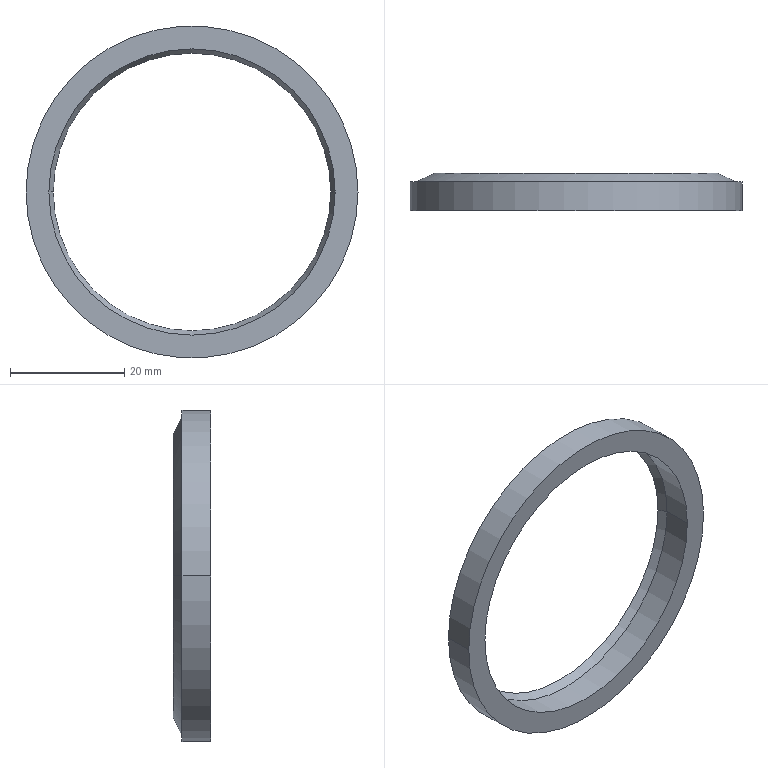Part | SolidWorks | features Revolution 1 | 1 solid | 11 faces | box 58 x 6.5 x 58 mm | volume 3817 mm3 | cone 4 | cylinder 4 | plane 3 | commonest cylinder face diameters 50 x2 58 x2
STEP:
#1=CARTESIAN_POINT('',(-24.25,6.5,0.));
#2=VERTEX_POINT('',#1);
#3=CARTESIAN_POINT('',(24.25,6.5,0.));
#4=VERTEX_POINT('',#3);
#5=CARTESIAN_POINT('',(0.,6.5,0.));
#6=DIRECTION('',(0.,-1.,0.));
#7=DIRECTION('',(1.,0.,0.));
#8=AXIS2_PLACEMENT_3D('',#5,#6,#7);
#9=CIRCLE('',#8,24.25);
#10=EDGE_CURVE('',#2,#4,#9,.T.);
#11=ORIENTED_EDGE('',*,*,#10,.F.);
#12=CARTESIAN_POINT('',(-25.,5.,0.));
#13=VERTEX_POINT('',#12);
#14=CARTESIAN_POINT('',(-24.25,6.5,0.));
#15=DIRECTION('',(-0.4472,-0.8944,0.));
#16=VECTOR('',#15,1000.);
#17=LINE('',#14,#16);
#18=EDGE_CURVE('',#2,#13,#17,.T.);
#19=ORIENTED_EDGE('',*,*,#18,.T.);
#20=CARTESIAN_POINT('',(25.,5.,0.));
#21=VERTEX_POINT('',#20);
#22=CARTESIAN_POINT('',(0.,5.,0.));
#23=DIRECTION('',(0.,-1.,0.));
#24=DIRECTION('',(1.,0.,0.));
#25=AXIS2_PLACEMENT_3D('',#22,#23,#24);
#26=CIRCLE('',#25,25.);
#27=EDGE_CURVE('',#13,#21,#26,.T.);
#28=ORIENTED_EDGE('',*,*,#27,.T.);
#29=CARTESIAN_POINT('',(24.25,6.5,0.));
#30=DIRECTION('',(0.4472,-0.8944,0.));
#31=VECTOR('',#30,1000.);
#32=LINE('',#29,#31);
#33=EDGE_CURVE('',#4,#21,#32,.T.);
#34=ORIENTED_EDGE('',*,*,#33,.F.);
#35=EDGE_LOOP('',(#11,#19,#28,#34));
#36=FACE_OUTER_BOUND('',#35,.T.);
#37=CARTESIAN_POINT('',(0.,6.5,0.));
#38=DIRECTION('',(0.,-1.,0.));
#39=DIRECTION('',(1.,0.,0.));
#40=AXIS2_PLACEMENT_3D('',#37,#38,#39);
#41=CONICAL_SURFACE('',#40,24.25,0.4636);
#42=ADVANCED_FACE('',(#36),#41,.F.);
#43=CARTESIAN_POINT('',(24.75,6.5,0.));
#44=VERTEX_POINT('',#43);
#45=CARTESIAN_POINT('',(-24.75,6.5,0.));
#46=VERTEX_POINT('',#45);
#47=CARTESIAN_POINT('',(0.,6.5,0.));
#48=DIRECTION('',(0.,-1.,0.));
#49=DIRECTION('',(1.,0.,0.));
#50=AXIS2_PLACEMENT_3D('',#47,#48,#49);
#51=CIRCLE('',#50,24.75);
#52=EDGE_CURVE('',#44,#46,#51,.T.);
#53=ORIENTED_EDGE('',*,*,#52,.T.);
#54=CARTESIAN_POINT('',(-28.,5.,0.));
#55=VERTEX_POINT('',#54);
#56=CARTESIAN_POINT('',(-28.,5.,0.));
#57=DIRECTION('',(-0.908,-0.4191,0.));
#58=VECTOR('',#57,1000.);
#59=LINE('',#56,#58);
#60=EDGE_CURVE('',#46,#55,#59,.T.);
#61=ORIENTED_EDGE('',*,*,#60,.T.);
#62=CARTESIAN_POINT('',(28.,5.,0.));
#63=VERTEX_POINT('',#62);
#64=CARTESIAN_POINT('',(0.,5.,0.));
#65=DIRECTION('',(0.,-1.,0.));
#66=DIRECTION('',(1.,0.,0.));
#67=AXIS2_PLACEMENT_3D('',#64,#65,#66);
#68=CIRCLE('',#67,28.);
#69=EDGE_CURVE('',#63,#55,#68,.T.);
#70=ORIENTED_EDGE('',*,*,#69,.F.);
#71=CARTESIAN_POINT('',(28.,5.,0.));
#72=DIRECTION('',(0.908,-0.4191,0.));
#73=VECTOR('',#72,1000.);
#74=LINE('',#71,#73);
#75=EDGE_CURVE('',#44,#63,#74,.T.);
#76=ORIENTED_EDGE('',*,*,#75,.F.);
#77=EDGE_LOOP('',(#53,#61,#70,#76));
#78=FACE_OUTER_BOUND('',#77,.T.);
#79=CARTESIAN_POINT('',(0.,5.,0.));
#80=DIRECTION('',(0.,-1.,0.));
#81=DIRECTION('',(1.,0.,0.));
#82=AXIS2_PLACEMENT_3D('',#79,#80,#81);
#83=CONICAL_SURFACE('',#82,28.,1.138);
#84=ADVANCED_FACE('',(#78),#83,.T.);
#85=CARTESIAN_POINT('',(29.,5.,0.));
#86=VERTEX_POINT('',#85);
#87=CARTESIAN_POINT('',(-29.,5.,0.));
#88=VERTEX_POINT('',#87);
#89=CARTESIAN_POINT('',(0.,5.,0.));
#90=DIRECTION('',(0.,-1.,0.));
#91=DIRECTION('',(1.,0.,0.));
#92=AXIS2_PLACEMENT_3D('',#89,#90,#91);
#93=CIRCLE('',#92,29.);
#94=EDGE_CURVE('',#86,#88,#93,.T.);
#95=ORIENTED_EDGE('',*,*,#94,.T.);
#96=CARTESIAN_POINT('',(-29.,0.,0.));
#97=VERTEX_POINT('',#96);
#98=CARTESIAN_POINT('',(-29.,-1000.,0.));
#99=DIRECTION('',(0.,-1.,0.));
#100=VECTOR('',#99,1000.);
#101=LINE('',#98,#100);
#102=EDGE_CURVE('',#88,#97,#101,.T.);
#103=ORIENTED_EDGE('',*,*,#102,.T.);
#104=CARTESIAN_POINT('',(29.,0.,0.));
#105=VERTEX_POINT('',#104);
#106=CARTESIAN_POINT('',(0.,0.,0.));
#107=DIRECTION('',(0.,-1.,0.));
#108=DIRECTION('',(1.,0.,0.));
#109=AXIS2_PLACEMENT_3D('',#106,#107,#108);
#110=CIRCLE('',#109,29.);
#111=EDGE_CURVE('',#105,#97,#110,.T.);
#112=ORIENTED_EDGE('',*,*,#111,.F.);
#113=CARTESIAN_POINT('',(29.,-1000.,0.));
#114=DIRECTION('',(0.,-1.,0.));
#115=VECTOR('',#114,1000.);
#116=LINE('',#113,#115);
#117=EDGE_CURVE('',#86,#105,#116,.T.);
#118=ORIENTED_EDGE('',*,*,#117,.F.);
#119=EDGE_LOOP('',(#95,#103,#112,#118));
#120=FACE_OUTER_BOUND('',#119,.T.);
#121=CARTESIAN_POINT('',(0.,-1000.,0.));
#122=DIRECTION('',(0.,-1.,0.));
#123=DIRECTION('',(1.,0.,0.));
#124=AXIS2_PLACEMENT_3D('',#121,#122,#123);
#125=CYLINDRICAL_SURFACE('',#124,29.);
#126=ADVANCED_FACE('',(#120),#125,.T.);
#127=ORIENTED_EDGE('',*,*,#27,.F.);
#128=CARTESIAN_POINT('',(-25.,0.,0.));
#129=VERTEX_POINT('',#128);
#130=CARTESIAN_POINT('',(-25.,-1000.,0.));
#131=DIRECTION('',(0.,-1.,0.));
#132=VECTOR('',#131,1000.);
#133=LINE('',#130,#132);
#134=EDGE_CURVE('',#13,#129,#133,.T.);
#135=ORIENTED_EDGE('',*,*,#134,.T.);
#136=CARTESIAN_POINT('',(25.,0.,0.));
#137=VERTEX_POINT('',#136);
#138=CARTESIAN_POINT('',(0.,0.,0.));
#139=DIRECTION('',(0.,-1.,0.));
#140=DIRECTION('',(1.,0.,0.));
#141=AXIS2_PLACEMENT_3D('',#138,#139,#140);
#142=CIRCLE('',#141,25.);
#143=EDGE_CURVE('',#129,#137,#142,.T.);
#144=ORIENTED_EDGE('',*,*,#143,.T.);
#145=CARTESIAN_POINT('',(25.,-1000.,0.));
#146=DIRECTION('',(0.,-1.,0.));
#147=VECTOR('',#146,1000.);
#148=LINE('',#145,#147);
#149=EDGE_CURVE('',#21,#137,#148,.T.);
#150=ORIENTED_EDGE('',*,*,#149,.F.);
#151=EDGE_LOOP('',(#127,#135,#144,#150));
#152=FACE_OUTER_BOUND('',#151,.T.);
#153=CARTESIAN_POINT('',(0.,-1000.,0.));
#154=DIRECTION('',(0.,-1.,0.));
#155=DIRECTION('',(1.,0.,0.));
#156=AXIS2_PLACEMENT_3D('',#153,#154,#155);
#157=CYLINDRICAL_SURFACE('',#156,25.);
#158=ADVANCED_FACE('',(#152),#157,.F.);
#159=ORIENTED_EDGE('',*,*,#134,.F.);
#160=CARTESIAN_POINT('',(0.,5.,0.));
#161=DIRECTION('',(0.,-1.,0.));
#162=DIRECTION('',(1.,0.,0.));
#163=AXIS2_PLACEMENT_3D('',#160,#161,#162);
#164=CIRCLE('',#163,25.);
#165=EDGE_CURVE('',#21,#13,#164,.T.);
#166=ORIENTED_EDGE('',*,*,#165,.F.);
#167=ORIENTED_EDGE('',*,*,#149,.T.);
#168=CARTESIAN_POINT('',(0.,0.,0.));
#169=DIRECTION('',(0.,-1.,0.));
#170=DIRECTION('',(1.,0.,0.));
#171=AXIS2_PLACEMENT_3D('',#168,#169,#170);
#172=CIRCLE('',#171,25.);
#173=EDGE_CURVE('',#137,#129,#172,.T.);
#174=ORIENTED_EDGE('',*,*,#173,.T.);
#175=EDGE_LOOP('',(#159,#166,#167,#174));
#176=FACE_OUTER_BOUND('',#175,.T.);
#177=CARTESIAN_POINT('',(0.,-1000.,0.));
#178=DIRECTION('',(0.,-1.,0.));
#179=DIRECTION('',(1.,0.,0.));
#180=AXIS2_PLACEMENT_3D('',#177,#178,#179);
#181=CYLINDRICAL_SURFACE('',#180,25.);
#182=ADVANCED_FACE('',(#176),#181,.F.);
#183=ORIENTED_EDGE('',*,*,#111,.T.);
#184=CARTESIAN_POINT('',(0.,0.,0.));
#185=DIRECTION('',(0.,-1.,0.));
#186=DIRECTION('',(1.,0.,0.));
#187=AXIS2_PLACEMENT_3D('',#184,#185,#186);
#188=CIRCLE('',#187,29.);
#189=EDGE_CURVE('',#97,#105,#188,.T.);
#190=ORIENTED_EDGE('',*,*,#189,.T.);
#191=EDGE_LOOP('',(#183,#190));
#192=FACE_OUTER_BOUND('',#191,.T.);
#193=ORIENTED_EDGE('',*,*,#173,.F.);
#194=ORIENTED_EDGE('',*,*,#143,.F.);
#195=EDGE_LOOP('',(#193,#194));
#196=FACE_BOUND('',#195,.T.);
#197=CARTESIAN_POINT('',(25.,0.,0.));
#198=DIRECTION('',(0.,-1.,0.));
#199=DIRECTION('',(1.,0.,0.));
#200=AXIS2_PLACEMENT_3D('',#197,#198,#199);
#201=PLANE('',#200);
#202=ADVANCED_FACE('',(#192,#196),#201,.T.);
#203=ORIENTED_EDGE('',*,*,#102,.F.);
#204=CARTESIAN_POINT('',(0.,5.,0.));
#205=DIRECTION('',(0.,-1.,0.));
#206=DIRECTION('',(1.,0.,0.));
#207=AXIS2_PLACEMENT_3D('',#204,#205,#206);
#208=CIRCLE('',#207,29.);
#209=EDGE_CURVE('',#88,#86,#208,.T.);
#210=ORIENTED_EDGE('',*,*,#209,.T.);
#211=ORIENTED_EDGE('',*,*,#117,.T.);
#212=ORIENTED_EDGE('',*,*,#189,.F.);
#213=EDGE_LOOP('',(#203,#210,#211,#212));
#214=FACE_OUTER_BOUND('',#213,.T.);
#215=CARTESIAN_POINT('',(0.,-1000.,0.));
#216=DIRECTION('',(0.,-1.,0.));
#217=DIRECTION('',(1.,0.,0.));
#218=AXIS2_PLACEMENT_3D('',#215,#216,#217);
#219=CYLINDRICAL_SURFACE('',#218,29.);
#220=ADVANCED_FACE('',(#214),#219,.T.);
#221=ORIENTED_EDGE('',*,*,#69,.T.);
#222=CARTESIAN_POINT('',(0.,5.,0.));
#223=DIRECTION('',(0.,-1.,0.));
#224=DIRECTION('',(1.,0.,0.));
#225=AXIS2_PLACEMENT_3D('',#222,#223,#224);
#226=CIRCLE('',#225,28.);
#227=EDGE_CURVE('',#55,#63,#226,.T.);
#228=ORIENTED_EDGE('',*,*,#227,.T.);
#229=EDGE_LOOP('',(#221,#228));
#230=FACE_BOUND('',#229,.T.);
#231=ORIENTED_EDGE('',*,*,#94,.F.);
#232=ORIENTED_EDGE('',*,*,#209,.F.);
#233=EDGE_LOOP('',(#231,#232));
#234=FACE_OUTER_BOUND('',#233,.T.);
#235=CARTESIAN_POINT('',(29.,5.,0.));
#236=DIRECTION('',(0.,1.,0.));
#237=DIRECTION('',(-1.,0.,0.));
#238=AXIS2_PLACEMENT_3D('',#235,#236,#237);
#239=PLANE('',#238);
#240=ADVANCED_FACE('',(#230,#234),#239,.T.);
#241=ORIENTED_EDGE('',*,*,#60,.F.);
#242=CARTESIAN_POINT('',(0.,6.5,0.));
#243=DIRECTION('',(0.,-1.,0.));
#244=DIRECTION('',(1.,0.,0.));
#245=AXIS2_PLACEMENT_3D('',#242,#243,#244);
#246=CIRCLE('',#245,24.75);
#247=EDGE_CURVE('',#46,#44,#246,.T.);
#248=ORIENTED_EDGE('',*,*,#247,.T.);
#249=ORIENTED_EDGE('',*,*,#75,.T.);
#250=ORIENTED_EDGE('',*,*,#227,.F.);
#251=EDGE_LOOP('',(#241,#248,#249,#250));
#252=FACE_OUTER_BOUND('',#251,.T.);
#253=CARTESIAN_POINT('',(0.,5.,0.));
#254=DIRECTION('',(0.,-1.,0.));
#255=DIRECTION('',(1.,0.,0.));
#256=AXIS2_PLACEMENT_3D('',#253,#254,#255);
#257=CONICAL_SURFACE('',#256,28.,1.138);
#258=ADVANCED_FACE('',(#252),#257,.T.);
#259=CARTESIAN_POINT('',(0.,6.5,0.));
#260=DIRECTION('',(0.,-1.,0.));
#261=DIRECTION('',(1.,0.,0.));
#262=AXIS2_PLACEMENT_3D('',#259,#260,#261);
#263=CIRCLE('',#262,24.25);
#264=EDGE_CURVE('',#4,#2,#263,.T.);
#265=ORIENTED_EDGE('',*,*,#264,.T.);
#266=ORIENTED_EDGE('',*,*,#10,.T.);
#267=EDGE_LOOP('',(#265,#266));
#268=FACE_BOUND('',#267,.T.);
#269=ORIENTED_EDGE('',*,*,#52,.F.);
#270=ORIENTED_EDGE('',*,*,#247,.F.);
#271=EDGE_LOOP('',(#269,#270));
#272=FACE_OUTER_BOUND('',#271,.T.);
#273=CARTESIAN_POINT('',(24.75,6.5,0.));
#274=DIRECTION('',(0.,1.,0.));
#275=DIRECTION('',(-1.,0.,0.));
#276=AXIS2_PLACEMENT_3D('',#273,#274,#275);
#277=PLANE('',#276);
#278=ADVANCED_FACE('',(#268,#272),#277,.T.);
#279=ORIENTED_EDGE('',*,*,#18,.F.);
#280=ORIENTED_EDGE('',*,*,#264,.F.);
#281=ORIENTED_EDGE('',*,*,#33,.T.);
#282=ORIENTED_EDGE('',*,*,#165,.T.);
#283=EDGE_LOOP('',(#279,#280,#281,#282));
#284=FACE_OUTER_BOUND('',#283,.T.);
#285=CARTESIAN_POINT('',(0.,6.5,0.));
#286=DIRECTION('',(0.,-1.,0.));
#287=DIRECTION('',(1.,0.,0.));
#288=AXIS2_PLACEMENT_3D('',#285,#286,#287);
#289=CONICAL_SURFACE('',#288,24.25,0.4636);
#290=ADVANCED_FACE('',(#284),#289,.F.);
#291=CLOSED_SHELL('',(#42,#84,#126,#158,#182,#202,#220,#240,#258,#278,#290));
#292=MANIFOLD_SOLID_BREP('',#291);
#293=CARTESIAN_POINT('',(0.,0.,0.));
#294=DIRECTION('',(0.,0.,1.));
#295=DIRECTION('',(1.,0.,0.));
#296=AXIS2_PLACEMENT_3D('',#293,#294,#295);
#297=(LENGTH_UNIT()NAMED_UNIT(*)SI_UNIT(.MILLI.,.METRE.));
#298=UNCERTAINTY_MEASURE_WITH_UNIT(LENGTH_MEASURE(0.00001),#297,'','');
#299=(NAMED_UNIT(*)PLANE_ANGLE_UNIT()SI_UNIT($,.RADIAN.));
#300=(NAMED_UNIT(*)SI_UNIT($,.STERADIAN.)SOLID_ANGLE_UNIT());
#301=(GEOMETRIC_REPRESENTATION_CONTEXT(3)GLOBAL_UNCERTAINTY_ASSIGNED_CONTEXT((#298))GLOBAL_UNIT_ASSIGNED_CONTEXT((#297,#299,#300))REPRESENTATION_CONTEXT('',''));
#302=ADVANCED_BREP_SHAPE_REPRESENTATION('',(#292,#296),#301);